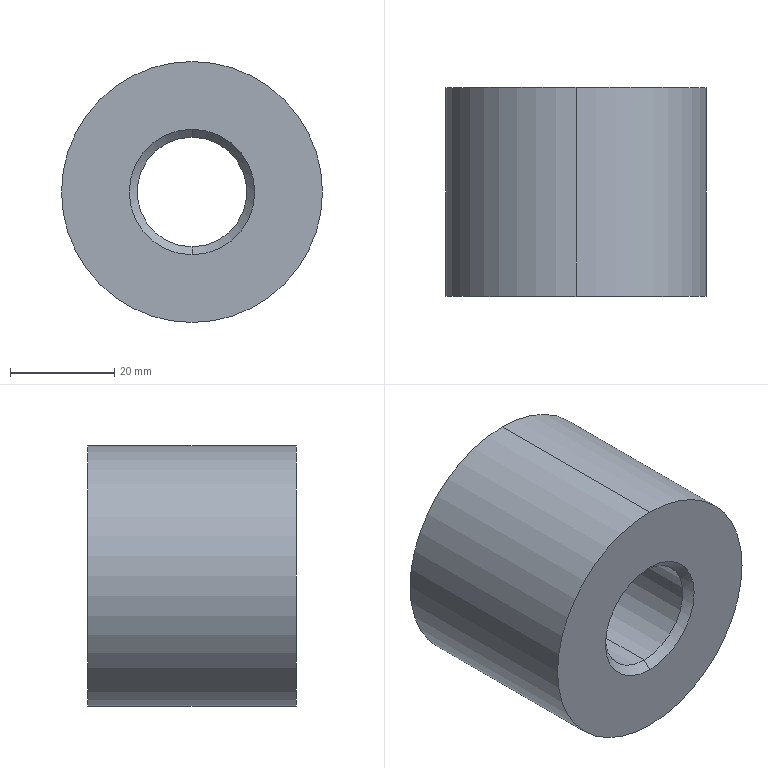Part | SolidWorks | features Extrusion 1, HoleWzd 1 | 1 solid | 8 faces | box 50 x 40 x 50 mm | volume 64605 mm3 | cylinder 4 | cone 2 | plane 2 | commonest cylinder face diameters 21 x2 50 x2
STEP:
#1=CARTESIAN_POINT('',(0.,1.525,10.5));
#2=VERTEX_POINT('',#1);
#3=CARTESIAN_POINT('',(0.,1.525,-10.5));
#4=VERTEX_POINT('',#3);
#5=CARTESIAN_POINT('',(0.,1.525,0.));
#6=DIRECTION('',(0.,-1.,0.));
#7=DIRECTION('',(0.,0.,-1.));
#8=AXIS2_PLACEMENT_3D('',#5,#6,#7);
#9=CIRCLE('',#8,10.5);
#10=EDGE_CURVE('',#2,#4,#9,.T.);
#11=ORIENTED_EDGE('',*,*,#10,.F.);
#12=CARTESIAN_POINT('',(0.,0.,12.025));
#13=VERTEX_POINT('',#12);
#14=CARTESIAN_POINT('',(0.,0.,12.025));
#15=DIRECTION('',(0.,-0.7071,0.7071));
#16=VECTOR('',#15,1000.);
#17=LINE('',#14,#16);
#18=EDGE_CURVE('',#2,#13,#17,.T.);
#19=ORIENTED_EDGE('',*,*,#18,.T.);
#20=CARTESIAN_POINT('',(0.,0.,-12.025));
#21=VERTEX_POINT('',#20);
#22=CARTESIAN_POINT('',(0.,0.,0.));
#23=DIRECTION('',(0.,-1.,0.));
#24=DIRECTION('',(0.,0.,-1.));
#25=AXIS2_PLACEMENT_3D('',#22,#23,#24);
#26=CIRCLE('',#25,12.025);
#27=EDGE_CURVE('',#13,#21,#26,.T.);
#28=ORIENTED_EDGE('',*,*,#27,.T.);
#29=CARTESIAN_POINT('',(0.,0.,-12.025));
#30=DIRECTION('',(0.,-0.7071,-0.7071));
#31=VECTOR('',#30,1000.);
#32=LINE('',#29,#31);
#33=EDGE_CURVE('',#4,#21,#32,.T.);
#34=ORIENTED_EDGE('',*,*,#33,.F.);
#35=EDGE_LOOP('',(#11,#19,#28,#34));
#36=FACE_OUTER_BOUND('',#35,.T.);
#37=CARTESIAN_POINT('',(0.,0.,0.));
#38=DIRECTION('',(0.,-1.,0.));
#39=DIRECTION('',(0.,0.,-1.));
#40=AXIS2_PLACEMENT_3D('',#37,#38,#39);
#41=CONICAL_SURFACE('',#40,12.025,0.7854);
#42=ADVANCED_FACE('',(#36),#41,.F.);
#43=CARTESIAN_POINT('',(0.,40.,10.5));
#44=VERTEX_POINT('',#43);
#45=CARTESIAN_POINT('',(0.,40.,-10.5));
#46=VERTEX_POINT('',#45);
#47=CARTESIAN_POINT('',(0.,40.,0.));
#48=DIRECTION('',(0.,-1.,0.));
#49=DIRECTION('',(0.,0.,-1.));
#50=AXIS2_PLACEMENT_3D('',#47,#48,#49);
#51=CIRCLE('',#50,10.5);
#52=EDGE_CURVE('',#44,#46,#51,.T.);
#53=ORIENTED_EDGE('',*,*,#52,.F.);
#54=CARTESIAN_POINT('',(0.,0.,10.5));
#55=DIRECTION('',(0.,-1.,0.));
#56=VECTOR('',#55,1000.);
#57=LINE('',#54,#56);
#58=EDGE_CURVE('',#44,#2,#57,.T.);
#59=ORIENTED_EDGE('',*,*,#58,.T.);
#60=ORIENTED_EDGE('',*,*,#10,.T.);
#61=CARTESIAN_POINT('',(0.,0.,-10.5));
#62=DIRECTION('',(0.,-1.,0.));
#63=VECTOR('',#62,1000.);
#64=LINE('',#61,#63);
#65=EDGE_CURVE('',#46,#4,#64,.T.);
#66=ORIENTED_EDGE('',*,*,#65,.F.);
#67=EDGE_LOOP('',(#53,#59,#60,#66));
#68=FACE_OUTER_BOUND('',#67,.T.);
#69=CARTESIAN_POINT('',(0.,0.,0.));
#70=DIRECTION('',(0.,-1.,0.));
#71=DIRECTION('',(0.,0.,-1.));
#72=AXIS2_PLACEMENT_3D('',#69,#70,#71);
#73=CYLINDRICAL_SURFACE('',#72,10.5);
#74=ADVANCED_FACE('',(#68),#73,.F.);
#75=CARTESIAN_POINT('',(0.,40.,25.));
#76=VERTEX_POINT('',#75);
#77=CARTESIAN_POINT('',(0.,40.,-25.));
#78=VERTEX_POINT('',#77);
#79=CARTESIAN_POINT('',(0.,40.,0.));
#80=DIRECTION('',(0.,1.,0.));
#81=DIRECTION('',(0.,0.,1.));
#82=AXIS2_PLACEMENT_3D('',#79,#80,#81);
#83=CIRCLE('',#82,25.);
#84=EDGE_CURVE('',#76,#78,#83,.T.);
#85=ORIENTED_EDGE('',*,*,#84,.F.);
#86=CARTESIAN_POINT('',(0.,0.,25.));
#87=VERTEX_POINT('',#86);
#88=CARTESIAN_POINT('',(0.,40.,25.));
#89=DIRECTION('',(0.,-1.,0.));
#90=VECTOR('',#89,1000.);
#91=LINE('',#88,#90);
#92=EDGE_CURVE('',#76,#87,#91,.T.);
#93=ORIENTED_EDGE('',*,*,#92,.T.);
#94=CARTESIAN_POINT('',(0.,0.,-25.));
#95=VERTEX_POINT('',#94);
#96=CARTESIAN_POINT('',(0.,0.,0.));
#97=DIRECTION('',(0.,1.,0.));
#98=DIRECTION('',(0.,0.,1.));
#99=AXIS2_PLACEMENT_3D('',#96,#97,#98);
#100=CIRCLE('',#99,25.);
#101=EDGE_CURVE('',#87,#95,#100,.T.);
#102=ORIENTED_EDGE('',*,*,#101,.T.);
#103=CARTESIAN_POINT('',(0.,40.,-25.));
#104=DIRECTION('',(0.,-1.,0.));
#105=VECTOR('',#104,1000.);
#106=LINE('',#103,#105);
#107=EDGE_CURVE('',#78,#95,#106,.T.);
#108=ORIENTED_EDGE('',*,*,#107,.F.);
#109=EDGE_LOOP('',(#85,#93,#102,#108));
#110=FACE_OUTER_BOUND('',#109,.T.);
#111=CARTESIAN_POINT('',(0.,40.,0.));
#112=DIRECTION('',(0.,-1.,0.));
#113=DIRECTION('',(0.,0.,-1.));
#114=AXIS2_PLACEMENT_3D('',#111,#112,#113);
#115=CYLINDRICAL_SURFACE('',#114,25.);
#116=ADVANCED_FACE('',(#110),#115,.T.);
#117=ORIENTED_EDGE('',*,*,#92,.F.);
#118=CARTESIAN_POINT('',(0.,40.,0.));
#119=DIRECTION('',(0.,1.,0.));
#120=DIRECTION('',(0.,0.,1.));
#121=AXIS2_PLACEMENT_3D('',#118,#119,#120);
#122=CIRCLE('',#121,25.);
#123=EDGE_CURVE('',#78,#76,#122,.T.);
#124=ORIENTED_EDGE('',*,*,#123,.F.);
#125=ORIENTED_EDGE('',*,*,#107,.T.);
#126=CARTESIAN_POINT('',(0.,0.,0.));
#127=DIRECTION('',(0.,1.,0.));
#128=DIRECTION('',(0.,0.,1.));
#129=AXIS2_PLACEMENT_3D('',#126,#127,#128);
#130=CIRCLE('',#129,25.);
#131=EDGE_CURVE('',#95,#87,#130,.T.);
#132=ORIENTED_EDGE('',*,*,#131,.T.);
#133=EDGE_LOOP('',(#117,#124,#125,#132));
#134=FACE_OUTER_BOUND('',#133,.T.);
#135=CARTESIAN_POINT('',(0.,40.,0.));
#136=DIRECTION('',(0.,-1.,0.));
#137=DIRECTION('',(0.,0.,-1.));
#138=AXIS2_PLACEMENT_3D('',#135,#136,#137);
#139=CYLINDRICAL_SURFACE('',#138,25.);
#140=ADVANCED_FACE('',(#134),#139,.T.);
#141=CARTESIAN_POINT('',(0.,40.,0.));
#142=DIRECTION('',(0.,-1.,0.));
#143=DIRECTION('',(0.,0.,-1.));
#144=AXIS2_PLACEMENT_3D('',#141,#142,#143);
#145=CIRCLE('',#144,10.5);
#146=EDGE_CURVE('',#46,#44,#145,.T.);
#147=ORIENTED_EDGE('',*,*,#146,.T.);
#148=ORIENTED_EDGE('',*,*,#52,.T.);
#149=EDGE_LOOP('',(#147,#148));
#150=FACE_BOUND('',#149,.T.);
#151=ORIENTED_EDGE('',*,*,#123,.T.);
#152=ORIENTED_EDGE('',*,*,#84,.T.);
#153=EDGE_LOOP('',(#151,#152));
#154=FACE_OUTER_BOUND('',#153,.T.);
#155=CARTESIAN_POINT('',(0.,40.,0.));
#156=DIRECTION('',(0.,1.,0.));
#157=DIRECTION('',(0.,0.,1.));
#158=AXIS2_PLACEMENT_3D('',#155,#156,#157);
#159=PLANE('',#158);
#160=ADVANCED_FACE('',(#150,#154),#159,.T.);
#161=CARTESIAN_POINT('',(0.,0.,0.));
#162=DIRECTION('',(0.,-1.,0.));
#163=DIRECTION('',(0.,0.,-1.));
#164=AXIS2_PLACEMENT_3D('',#161,#162,#163);
#165=CIRCLE('',#164,12.025);
#166=EDGE_CURVE('',#21,#13,#165,.T.);
#167=ORIENTED_EDGE('',*,*,#166,.F.);
#168=ORIENTED_EDGE('',*,*,#27,.F.);
#169=EDGE_LOOP('',(#167,#168));
#170=FACE_BOUND('',#169,.T.);
#171=ORIENTED_EDGE('',*,*,#131,.F.);
#172=ORIENTED_EDGE('',*,*,#101,.F.);
#173=EDGE_LOOP('',(#171,#172));
#174=FACE_OUTER_BOUND('',#173,.T.);
#175=CARTESIAN_POINT('',(0.,0.,0.));
#176=DIRECTION('',(0.,1.,0.));
#177=DIRECTION('',(0.,0.,1.));
#178=AXIS2_PLACEMENT_3D('',#175,#176,#177);
#179=PLANE('',#178);
#180=ADVANCED_FACE('',(#170,#174),#179,.F.);
#181=ORIENTED_EDGE('',*,*,#58,.F.);
#182=ORIENTED_EDGE('',*,*,#146,.F.);
#183=ORIENTED_EDGE('',*,*,#65,.T.);
#184=CARTESIAN_POINT('',(0.,1.525,0.));
#185=DIRECTION('',(0.,-1.,0.));
#186=DIRECTION('',(0.,0.,-1.));
#187=AXIS2_PLACEMENT_3D('',#184,#185,#186);
#188=CIRCLE('',#187,10.5);
#189=EDGE_CURVE('',#4,#2,#188,.T.);
#190=ORIENTED_EDGE('',*,*,#189,.T.);
#191=EDGE_LOOP('',(#181,#182,#183,#190));
#192=FACE_OUTER_BOUND('',#191,.T.);
#193=CARTESIAN_POINT('',(0.,0.,0.));
#194=DIRECTION('',(0.,-1.,0.));
#195=DIRECTION('',(0.,0.,-1.));
#196=AXIS2_PLACEMENT_3D('',#193,#194,#195);
#197=CYLINDRICAL_SURFACE('',#196,10.5);
#198=ADVANCED_FACE('',(#192),#197,.F.);
#199=ORIENTED_EDGE('',*,*,#18,.F.);
#200=ORIENTED_EDGE('',*,*,#189,.F.);
#201=ORIENTED_EDGE('',*,*,#33,.T.);
#202=ORIENTED_EDGE('',*,*,#166,.T.);
#203=EDGE_LOOP('',(#199,#200,#201,#202));
#204=FACE_OUTER_BOUND('',#203,.T.);
#205=CARTESIAN_POINT('',(0.,0.,0.));
#206=DIRECTION('',(0.,-1.,0.));
#207=DIRECTION('',(0.,0.,-1.));
#208=AXIS2_PLACEMENT_3D('',#205,#206,#207);
#209=CONICAL_SURFACE('',#208,12.025,0.7854);
#210=ADVANCED_FACE('',(#204),#209,.F.);
#211=CLOSED_SHELL('',(#42,#74,#116,#140,#160,#180,#198,#210));
#212=MANIFOLD_SOLID_BREP('',#211);
#213=CARTESIAN_POINT('',(0.,0.,0.));
#214=DIRECTION('',(0.,0.,1.));
#215=DIRECTION('',(1.,0.,0.));
#216=AXIS2_PLACEMENT_3D('',#213,#214,#215);
#217=(LENGTH_UNIT()NAMED_UNIT(*)SI_UNIT(.MILLI.,.METRE.));
#218=UNCERTAINTY_MEASURE_WITH_UNIT(LENGTH_MEASURE(0.00001),#217,'','');
#219=(NAMED_UNIT(*)PLANE_ANGLE_UNIT()SI_UNIT($,.RADIAN.));
#220=(NAMED_UNIT(*)SI_UNIT($,.STERADIAN.)SOLID_ANGLE_UNIT());
#221=(GEOMETRIC_REPRESENTATION_CONTEXT(3)GLOBAL_UNCERTAINTY_ASSIGNED_CONTEXT((#218))GLOBAL_UNIT_ASSIGNED_CONTEXT((#217,#219,#220))REPRESENTATION_CONTEXT('',''));
#222=ADVANCED_BREP_SHAPE_REPRESENTATION('',(#212,#216),#221);